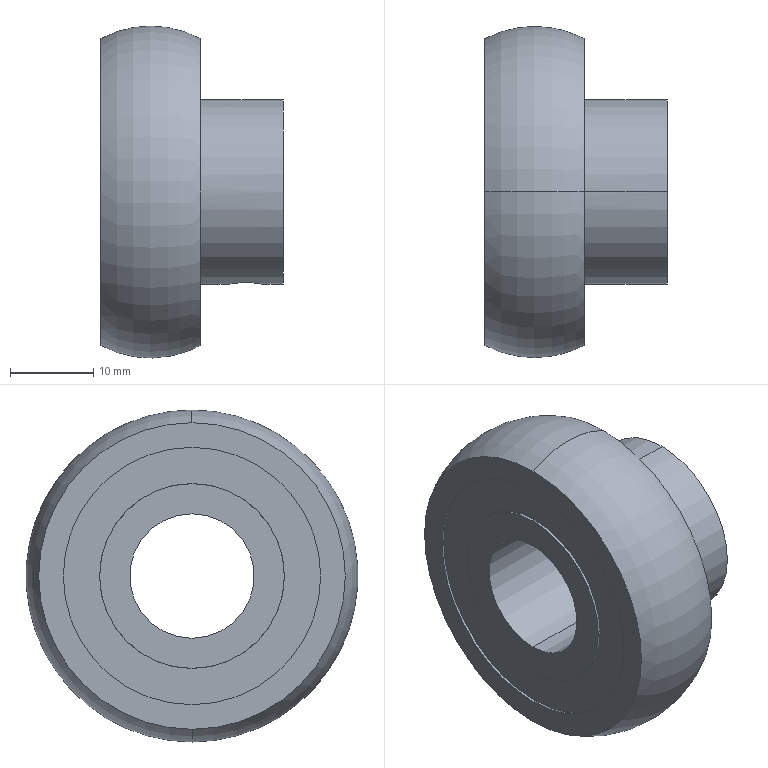Part | SolidWorks | features Revolution 3, RevCut 2, CirPattern 1 | 1 solid | 37 faces | box 22 x 40 x 40 mm | volume 10628 mm3 | cylinder 18 | plane 9 | sphere 8 | torus 2 | commonest cylinder face diameters 31 x6 22.27 x4 2 x2 4.307 x2 15 x2 22.25 x2